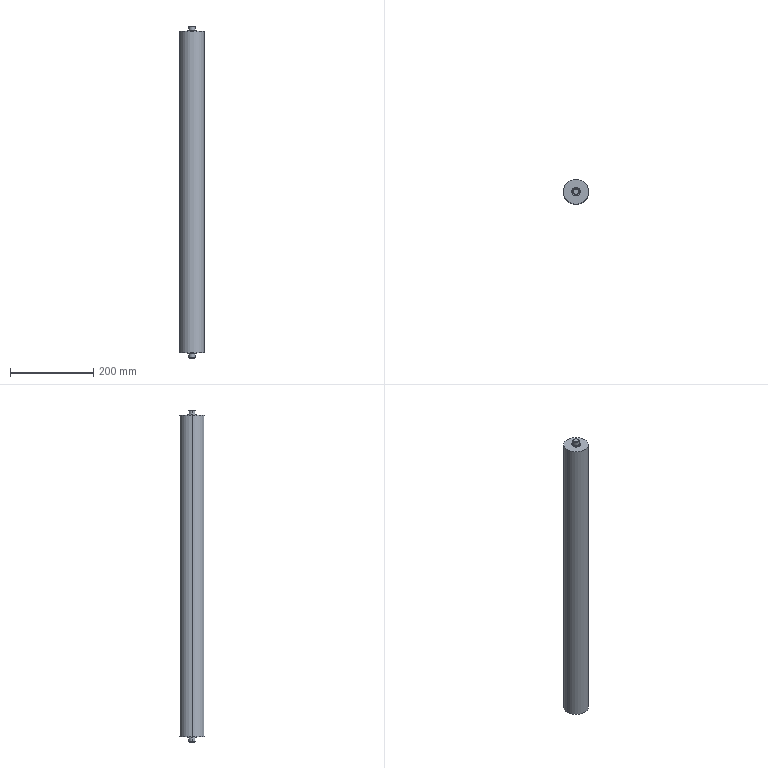Part | STEP file | Auxiliary roller 3 | 1 solid | 20 faces | box 60 x 60 x 799 mm | volume 2193510 mm3 | cylinder 10 | plane 6 | cone 4 | commonest cylinder face diameters 15 x4 20 x4 60 x2
STEP:
#1=CARTESIAN_POINT('',(0.,0.,0.));
#2=DIRECTION('',(0.,0.,1.));
#3=DIRECTION('',(1.,0.,0.));
#4=AXIS2_PLACEMENT_3D('',#1,#2,#3);
#5=CARTESIAN_POINT('',(30.,0.,0.));
#6=VERTEX_POINT('',#5);
#7=CARTESIAN_POINT('',(-30.,0.,0.));
#8=VERTEX_POINT('',#7);
#9=CARTESIAN_POINT('',(0.,0.,0.));
#10=DIRECTION('',(0.,0.,1.));
#11=DIRECTION('',(1.,0.,0.));
#12=AXIS2_PLACEMENT_3D('',#9,#10,#11);
#13=CIRCLE('',#12,30.);
#14=CARTESIAN_POINT('',(0.,0.,0.));
#15=DIRECTION('',(0.,0.,1.));
#16=DIRECTION('',(1.,0.,0.));
#17=AXIS2_PLACEMENT_3D('',#14,#15,#16);
#18=CYLINDRICAL_SURFACE('',#17,30.);
#19=CARTESIAN_POINT('',(0.,0.));
#20=DIRECTION('',(1.,0.));
#21=VECTOR('',#20,1.);
#22=LINE('',#19,#21);
#23=(GEOMETRIC_REPRESENTATION_CONTEXT(2)PARAMETRIC_REPRESENTATION_CONTEXT()REPRESENTATION_CONTEXT('',''));
#24=DEFINITIONAL_REPRESENTATION('',(#22),#23);
#25=PCURVE('',#18,#24);
#26=CARTESIAN_POINT('',(0.,0.,0.));
#27=DIRECTION('',(0.,0.,-1.));
#28=DIRECTION('',(-1.,0.,0.));
#29=AXIS2_PLACEMENT_3D('',#26,#27,#28);
#30=PLANE('',#29);
#31=CARTESIAN_POINT('',(-30.,0.));
#32=CARTESIAN_POINT('',(-30.,51.962));
#33=CARTESIAN_POINT('',(15.,25.981));
#34=CARTESIAN_POINT('',(60.,0.));
#35=CARTESIAN_POINT('',(15.,-25.981));
#36=CARTESIAN_POINT('',(-30.,-51.962));
#37=CARTESIAN_POINT('',(-30.,0.));
#38=(BOUNDED_CURVE()B_SPLINE_CURVE(2,(#31,#32,#33,#34,#35,#36,#37),.UNSPECIFIED.,.T.,.F.)B_SPLINE_CURVE_WITH_KNOTS((1,2,2,2,2,1),(-2.094,0.,2.094,4.189,6.283,8.378),.UNSPECIFIED.)CURVE()GEOMETRIC_REPRESENTATION_ITEM()RATIONAL_B_SPLINE_CURVE((1.,0.5,1.,0.5,1.,0.5,1.))REPRESENTATION_ITEM(''));
#39=(GEOMETRIC_REPRESENTATION_CONTEXT(2)PARAMETRIC_REPRESENTATION_CONTEXT()REPRESENTATION_CONTEXT('',''));
#40=DEFINITIONAL_REPRESENTATION('',(#38),#39);
#41=PCURVE('',#30,#40);
#42=SURFACE_CURVE('',#13,(#25,#41),.PCURVE_S1.);
#43=EDGE_CURVE('',#6,#8,#42,.T.);
#44=ORIENTED_EDGE('',*,*,#43,.T.);
#45=CARTESIAN_POINT('',(-30.,0.,774.));
#46=VERTEX_POINT('',#45);
#47=CARTESIAN_POINT('',(-30.,0.,0.));
#48=DIRECTION('',(0.,0.,1.));
#49=VECTOR('',#48,1.);
#50=LINE('',#47,#49);
#51=CARTESIAN_POINT('',(3.142,0.));
#52=DIRECTION('',(0.,1.));
#53=VECTOR('',#52,1.);
#54=LINE('',#51,#53);
#55=(GEOMETRIC_REPRESENTATION_CONTEXT(2)PARAMETRIC_REPRESENTATION_CONTEXT()REPRESENTATION_CONTEXT('',''));
#56=DEFINITIONAL_REPRESENTATION('',(#54),#55);
#57=PCURVE('',#18,#56);
#58=CARTESIAN_POINT('',(0.,0.,0.));
#59=DIRECTION('',(0.,0.,1.));
#60=DIRECTION('',(1.,0.,0.));
#61=AXIS2_PLACEMENT_3D('',#58,#59,#60);
#62=CYLINDRICAL_SURFACE('',#61,30.);
#63=CARTESIAN_POINT('',(3.142,0.));
#64=DIRECTION('',(0.,1.));
#65=VECTOR('',#64,1.);
#66=LINE('',#63,#65);
#67=(GEOMETRIC_REPRESENTATION_CONTEXT(2)PARAMETRIC_REPRESENTATION_CONTEXT()REPRESENTATION_CONTEXT('',''));
#68=DEFINITIONAL_REPRESENTATION('',(#66),#67);
#69=PCURVE('',#62,#68);
#70=SURFACE_CURVE('',#50,(#57,#69),.PCURVE_S1.);
#71=EDGE_CURVE('',#8,#46,#70,.T.);
#72=ORIENTED_EDGE('',*,*,#71,.T.);
#73=CARTESIAN_POINT('',(30.,0.,774.));
#74=VERTEX_POINT('',#73);
#75=CARTESIAN_POINT('',(0.,0.,774.));
#76=DIRECTION('',(0.,0.,-1.));
#77=DIRECTION('',(1.,0.,0.));
#78=AXIS2_PLACEMENT_3D('',#75,#76,#77);
#79=CIRCLE('',#78,30.);
#80=CARTESIAN_POINT('',(6.283,774.));
#81=DIRECTION('',(-1.,0.));
#82=VECTOR('',#81,1.);
#83=LINE('',#80,#82);
#84=(GEOMETRIC_REPRESENTATION_CONTEXT(2)PARAMETRIC_REPRESENTATION_CONTEXT()REPRESENTATION_CONTEXT('',''));
#85=DEFINITIONAL_REPRESENTATION('',(#83),#84);
#86=PCURVE('',#18,#85);
#87=CARTESIAN_POINT('',(0.,0.,774.));
#88=DIRECTION('',(0.,0.,-1.));
#89=DIRECTION('',(-1.,0.,0.));
#90=AXIS2_PLACEMENT_3D('',#87,#88,#89);
#91=PLANE('',#90);
#92=CARTESIAN_POINT('',(0.,0.));
#93=DIRECTION('',(-1.,0.));
#94=AXIS2_PLACEMENT_2D('',#92,#93);
#95=CIRCLE('',#94,30.);
#96=(GEOMETRIC_REPRESENTATION_CONTEXT(2)PARAMETRIC_REPRESENTATION_CONTEXT()REPRESENTATION_CONTEXT('',''));
#97=DEFINITIONAL_REPRESENTATION('',(#95),#96);
#98=PCURVE('',#91,#97);
#99=SURFACE_CURVE('',#79,(#86,#98),.PCURVE_S1.);
#100=EDGE_CURVE('',#46,#74,#99,.T.);
#101=ORIENTED_EDGE('',*,*,#100,.T.);
#102=CARTESIAN_POINT('',(30.,0.,0.));
#103=DIRECTION('',(0.,0.,1.));
#104=VECTOR('',#103,1.);
#105=LINE('',#102,#104);
#106=CARTESIAN_POINT('',(0.,0.));
#107=DIRECTION('',(0.,1.));
#108=VECTOR('',#107,1.);
#109=LINE('',#106,#108);
#110=(GEOMETRIC_REPRESENTATION_CONTEXT(2)PARAMETRIC_REPRESENTATION_CONTEXT()REPRESENTATION_CONTEXT('',''));
#111=DEFINITIONAL_REPRESENTATION('',(#109),#110);
#112=PCURVE('',#18,#111);
#113=CARTESIAN_POINT('',(6.283,0.));
#114=DIRECTION('',(0.,1.));
#115=VECTOR('',#114,1.);
#116=LINE('',#113,#115);
#117=(GEOMETRIC_REPRESENTATION_CONTEXT(2)PARAMETRIC_REPRESENTATION_CONTEXT()REPRESENTATION_CONTEXT('',''));
#118=DEFINITIONAL_REPRESENTATION('',(#116),#117);
#119=PCURVE('',#62,#118);
#120=SURFACE_CURVE('',#105,(#112,#119),.PCURVE_S1.);
#121=EDGE_CURVE('',#6,#74,#120,.T.);
#122=ORIENTED_EDGE('',*,*,#121,.F.);
#123=EDGE_LOOP('',(#44,#72,#101,#122));
#124=FACE_BOUND('',#123,.T.);
#125=ADVANCED_FACE('',(#124),#18,.T.);
#126=CARTESIAN_POINT('',(10.,0.,-2.5));
#127=VERTEX_POINT('',#126);
#128=CARTESIAN_POINT('',(-10.,0.,-2.5));
#129=VERTEX_POINT('',#128);
#130=CARTESIAN_POINT('',(0.,0.,-2.5));
#131=DIRECTION('',(0.,0.,1.));
#132=DIRECTION('',(1.,0.,0.));
#133=AXIS2_PLACEMENT_3D('',#130,#131,#132);
#134=CIRCLE('',#133,10.);
#135=CARTESIAN_POINT('',(0.,0.,0.));
#136=DIRECTION('',(0.,0.,1.));
#137=DIRECTION('',(1.,0.,0.));
#138=AXIS2_PLACEMENT_3D('',#135,#136,#137);
#139=CYLINDRICAL_SURFACE('',#138,10.);
#140=CARTESIAN_POINT('',(0.,-2.5));
#141=DIRECTION('',(1.,0.));
#142=VECTOR('',#141,1.);
#143=LINE('',#140,#142);
#144=(GEOMETRIC_REPRESENTATION_CONTEXT(2)PARAMETRIC_REPRESENTATION_CONTEXT()REPRESENTATION_CONTEXT('',''));
#145=DEFINITIONAL_REPRESENTATION('',(#143),#144);
#146=PCURVE('',#139,#145);
#147=CARTESIAN_POINT('',(0.,0.,-2.5));
#148=DIRECTION('',(0.,0.,-1.));
#149=DIRECTION('',(-1.,0.,0.));
#150=AXIS2_PLACEMENT_3D('',#147,#148,#149);
#151=PLANE('',#150);
#152=CARTESIAN_POINT('',(-10.,0.));
#153=CARTESIAN_POINT('',(-10.,17.321));
#154=CARTESIAN_POINT('',(5.,8.66));
#155=CARTESIAN_POINT('',(20.,0.));
#156=CARTESIAN_POINT('',(5.,-8.66));
#157=CARTESIAN_POINT('',(-10.,-17.321));
#158=CARTESIAN_POINT('',(-10.,0.));
#159=(BOUNDED_CURVE()B_SPLINE_CURVE(2,(#152,#153,#154,#155,#156,#157,#158),.UNSPECIFIED.,.T.,.F.)B_SPLINE_CURVE_WITH_KNOTS((1,2,2,2,2,1),(-2.094,0.,2.094,4.189,6.283,8.378),.UNSPECIFIED.)CURVE()GEOMETRIC_REPRESENTATION_ITEM()RATIONAL_B_SPLINE_CURVE((1.,0.5,1.,0.5,1.,0.5,1.))REPRESENTATION_ITEM(''));
#160=(GEOMETRIC_REPRESENTATION_CONTEXT(2)PARAMETRIC_REPRESENTATION_CONTEXT()REPRESENTATION_CONTEXT('',''));
#161=DEFINITIONAL_REPRESENTATION('',(#159),#160);
#162=PCURVE('',#151,#161);
#163=SURFACE_CURVE('',#134,(#146,#162),.PCURVE_S1.);
#164=EDGE_CURVE('',#127,#129,#163,.T.);
#165=ORIENTED_EDGE('',*,*,#164,.T.);
#166=CARTESIAN_POINT('',(-10.,0.,0.));
#167=VERTEX_POINT('',#166);
#168=CARTESIAN_POINT('',(-10.,0.,0.));
#169=DIRECTION('',(0.,0.,1.));
#170=VECTOR('',#169,1.);
#171=LINE('',#168,#170);
#172=CARTESIAN_POINT('',(3.142,0.));
#173=DIRECTION('',(0.,1.));
#174=VECTOR('',#173,1.);
#175=LINE('',#172,#174);
#176=(GEOMETRIC_REPRESENTATION_CONTEXT(2)PARAMETRIC_REPRESENTATION_CONTEXT()REPRESENTATION_CONTEXT('',''));
#177=DEFINITIONAL_REPRESENTATION('',(#175),#176);
#178=PCURVE('',#139,#177);
#179=CARTESIAN_POINT('',(0.,0.,0.));
#180=DIRECTION('',(0.,0.,1.));
#181=DIRECTION('',(1.,0.,0.));
#182=AXIS2_PLACEMENT_3D('',#179,#180,#181);
#183=CYLINDRICAL_SURFACE('',#182,10.);
#184=CARTESIAN_POINT('',(3.142,0.));
#185=DIRECTION('',(0.,1.));
#186=VECTOR('',#185,1.);
#187=LINE('',#184,#186);
#188=(GEOMETRIC_REPRESENTATION_CONTEXT(2)PARAMETRIC_REPRESENTATION_CONTEXT()REPRESENTATION_CONTEXT('',''));
#189=DEFINITIONAL_REPRESENTATION('',(#187),#188);
#190=PCURVE('',#183,#189);
#191=SURFACE_CURVE('',#171,(#178,#190),.PCURVE_S1.);
#192=EDGE_CURVE('',#129,#167,#191,.T.);
#193=ORIENTED_EDGE('',*,*,#192,.T.);
#194=CARTESIAN_POINT('',(10.,0.,0.));
#195=VERTEX_POINT('',#194);
#196=CARTESIAN_POINT('',(0.,0.,0.));
#197=DIRECTION('',(0.,0.,1.));
#198=DIRECTION('',(1.,0.,0.));
#199=AXIS2_PLACEMENT_3D('',#196,#197,#198);
#200=CIRCLE('',#199,10.);
#201=CARTESIAN_POINT('',(0.,0.));
#202=DIRECTION('',(1.,0.));
#203=VECTOR('',#202,1.);
#204=LINE('',#201,#203);
#205=(GEOMETRIC_REPRESENTATION_CONTEXT(2)PARAMETRIC_REPRESENTATION_CONTEXT()REPRESENTATION_CONTEXT('',''));
#206=DEFINITIONAL_REPRESENTATION('',(#204),#205);
#207=PCURVE('',#139,#206);
#208=CARTESIAN_POINT('',(-10.,0.));
#209=CARTESIAN_POINT('',(-10.,17.321));
#210=CARTESIAN_POINT('',(5.,8.66));
#211=CARTESIAN_POINT('',(20.,0.));
#212=CARTESIAN_POINT('',(5.,-8.66));
#213=CARTESIAN_POINT('',(-10.,-17.321));
#214=CARTESIAN_POINT('',(-10.,0.));
#215=(BOUNDED_CURVE()B_SPLINE_CURVE(2,(#208,#209,#210,#211,#212,#213,#214),.UNSPECIFIED.,.T.,.F.)B_SPLINE_CURVE_WITH_KNOTS((1,2,2,2,2,1),(-2.094,0.,2.094,4.189,6.283,8.378),.UNSPECIFIED.)CURVE()GEOMETRIC_REPRESENTATION_ITEM()RATIONAL_B_SPLINE_CURVE((1.,0.5,1.,0.5,1.,0.5,1.))REPRESENTATION_ITEM(''));
#216=(GEOMETRIC_REPRESENTATION_CONTEXT(2)PARAMETRIC_REPRESENTATION_CONTEXT()REPRESENTATION_CONTEXT('',''));
#217=DEFINITIONAL_REPRESENTATION('',(#215),#216);
#218=PCURVE('',#30,#217);
#219=SURFACE_CURVE('',#200,(#207,#218),.PCURVE_S1.);
#220=EDGE_CURVE('',#195,#167,#219,.T.);
#221=ORIENTED_EDGE('',*,*,#220,.F.);
#222=CARTESIAN_POINT('',(10.,0.,0.));
#223=DIRECTION('',(0.,0.,1.));
#224=VECTOR('',#223,1.);
#225=LINE('',#222,#224);
#226=CARTESIAN_POINT('',(0.,0.));
#227=DIRECTION('',(0.,1.));
#228=VECTOR('',#227,1.);
#229=LINE('',#226,#228);
#230=(GEOMETRIC_REPRESENTATION_CONTEXT(2)PARAMETRIC_REPRESENTATION_CONTEXT()REPRESENTATION_CONTEXT('',''));
#231=DEFINITIONAL_REPRESENTATION('',(#229),#230);
#232=PCURVE('',#139,#231);
#233=CARTESIAN_POINT('',(6.283,0.));
#234=DIRECTION('',(0.,1.));
#235=VECTOR('',#234,1.);
#236=LINE('',#233,#235);
#237=(GEOMETRIC_REPRESENTATION_CONTEXT(2)PARAMETRIC_REPRESENTATION_CONTEXT()REPRESENTATION_CONTEXT('',''));
#238=DEFINITIONAL_REPRESENTATION('',(#236),#237);
#239=PCURVE('',#183,#238);
#240=SURFACE_CURVE('',#225,(#232,#239),.PCURVE_S1.);
#241=EDGE_CURVE('',#127,#195,#240,.T.);
#242=ORIENTED_EDGE('',*,*,#241,.F.);
#243=EDGE_LOOP('',(#165,#193,#221,#242));
#244=FACE_BOUND('',#243,.T.);
#245=ADVANCED_FACE('',(#244),#139,.T.);
#246=CARTESIAN_POINT('',(10.,0.,774.));
#247=VERTEX_POINT('',#246);
#248=CARTESIAN_POINT('',(-10.,0.,774.));
#249=VERTEX_POINT('',#248);
#250=CARTESIAN_POINT('',(0.,0.,774.));
#251=DIRECTION('',(0.,0.,1.));
#252=DIRECTION('',(1.,0.,0.));
#253=AXIS2_PLACEMENT_3D('',#250,#251,#252);
#254=CIRCLE('',#253,10.);
#255=CARTESIAN_POINT('',(0.,0.,774.));
#256=DIRECTION('',(0.,0.,1.));
#257=DIRECTION('',(1.,0.,0.));
#258=AXIS2_PLACEMENT_3D('',#255,#256,#257);
#259=CYLINDRICAL_SURFACE('',#258,10.);
#260=CARTESIAN_POINT('',(0.,0.));
#261=DIRECTION('',(1.,0.));
#262=VECTOR('',#261,1.);
#263=LINE('',#260,#262);
#264=(GEOMETRIC_REPRESENTATION_CONTEXT(2)PARAMETRIC_REPRESENTATION_CONTEXT()REPRESENTATION_CONTEXT('',''));
#265=DEFINITIONAL_REPRESENTATION('',(#263),#264);
#266=PCURVE('',#259,#265);
#267=CARTESIAN_POINT('',(-10.,0.));
#268=CARTESIAN_POINT('',(-10.,17.321));
#269=CARTESIAN_POINT('',(5.,8.66));
#270=CARTESIAN_POINT('',(20.,0.));
#271=CARTESIAN_POINT('',(5.,-8.66));
#272=CARTESIAN_POINT('',(-10.,-17.321));
#273=CARTESIAN_POINT('',(-10.,0.));
#274=(BOUNDED_CURVE()B_SPLINE_CURVE(2,(#267,#268,#269,#270,#271,#272,#273),.UNSPECIFIED.,.T.,.F.)B_SPLINE_CURVE_WITH_KNOTS((1,2,2,2,2,1),(-2.094,0.,2.094,4.189,6.283,8.378),.UNSPECIFIED.)CURVE()GEOMETRIC_REPRESENTATION_ITEM()RATIONAL_B_SPLINE_CURVE((1.,0.5,1.,0.5,1.,0.5,1.))REPRESENTATION_ITEM(''));
#275=(GEOMETRIC_REPRESENTATION_CONTEXT(2)PARAMETRIC_REPRESENTATION_CONTEXT()REPRESENTATION_CONTEXT('',''));
#276=DEFINITIONAL_REPRESENTATION('',(#274),#275);
#277=PCURVE('',#91,#276);
#278=SURFACE_CURVE('',#254,(#266,#277),.PCURVE_S1.);
#279=EDGE_CURVE('',#247,#249,#278,.T.);
#280=ORIENTED_EDGE('',*,*,#279,.T.);
#281=CARTESIAN_POINT('',(-10.,0.,776.5));
#282=VERTEX_POINT('',#281);
#283=CARTESIAN_POINT('',(-10.,0.,774.));
#284=DIRECTION('',(0.,0.,1.));
#285=VECTOR('',#284,1.);
#286=LINE('',#283,#285);
#287=CARTESIAN_POINT('',(3.142,0.));
#288=DIRECTION('',(0.,1.));
#289=VECTOR('',#288,1.);
#290=LINE('',#287,#289);
#291=(GEOMETRIC_REPRESENTATION_CONTEXT(2)PARAMETRIC_REPRESENTATION_CONTEXT()REPRESENTATION_CONTEXT('',''));
#292=DEFINITIONAL_REPRESENTATION('',(#290),#291);
#293=PCURVE('',#259,#292);
#294=CARTESIAN_POINT('',(0.,0.,774.));
#295=DIRECTION('',(0.,0.,1.));
#296=DIRECTION('',(1.,0.,0.));
#297=AXIS2_PLACEMENT_3D('',#294,#295,#296);
#298=CYLINDRICAL_SURFACE('',#297,10.);
#299=CARTESIAN_POINT('',(3.142,0.));
#300=DIRECTION('',(0.,1.));
#301=VECTOR('',#300,1.);
#302=LINE('',#299,#301);
#303=(GEOMETRIC_REPRESENTATION_CONTEXT(2)PARAMETRIC_REPRESENTATION_CONTEXT()REPRESENTATION_CONTEXT('',''));
#304=DEFINITIONAL_REPRESENTATION('',(#302),#303);
#305=PCURVE('',#298,#304);
#306=SURFACE_CURVE('',#286,(#293,#305),.PCURVE_S1.);
#307=EDGE_CURVE('',#249,#282,#306,.T.);
#308=ORIENTED_EDGE('',*,*,#307,.T.);
#309=CARTESIAN_POINT('',(10.,0.,776.5));
#310=VERTEX_POINT('',#309);
#311=CARTESIAN_POINT('',(0.,0.,776.5));
#312=DIRECTION('',(0.,0.,-1.));
#313=DIRECTION('',(1.,0.,0.));
#314=AXIS2_PLACEMENT_3D('',#311,#312,#313);
#315=CIRCLE('',#314,10.);
#316=CARTESIAN_POINT('',(6.283,2.5));
#317=DIRECTION('',(-1.,0.));
#318=VECTOR('',#317,1.);
#319=LINE('',#316,#318);
#320=(GEOMETRIC_REPRESENTATION_CONTEXT(2)PARAMETRIC_REPRESENTATION_CONTEXT()REPRESENTATION_CONTEXT('',''));
#321=DEFINITIONAL_REPRESENTATION('',(#319),#320);
#322=PCURVE('',#259,#321);
#323=CARTESIAN_POINT('',(0.,0.,776.5));
#324=DIRECTION('',(0.,0.,-1.));
#325=DIRECTION('',(-1.,0.,0.));
#326=AXIS2_PLACEMENT_3D('',#323,#324,#325);
#327=PLANE('',#326);
#328=CARTESIAN_POINT('',(0.,0.));
#329=DIRECTION('',(-1.,0.));
#330=AXIS2_PLACEMENT_2D('',#328,#329);
#331=CIRCLE('',#330,10.);
#332=(GEOMETRIC_REPRESENTATION_CONTEXT(2)PARAMETRIC_REPRESENTATION_CONTEXT()REPRESENTATION_CONTEXT('',''));
#333=DEFINITIONAL_REPRESENTATION('',(#331),#332);
#334=PCURVE('',#327,#333);
#335=SURFACE_CURVE('',#315,(#322,#334),.PCURVE_S1.);
#336=EDGE_CURVE('',#282,#310,#335,.T.);
#337=ORIENTED_EDGE('',*,*,#336,.T.);
#338=CARTESIAN_POINT('',(10.,0.,774.));
#339=DIRECTION('',(0.,0.,1.));
#340=VECTOR('',#339,1.);
#341=LINE('',#338,#340);
#342=CARTESIAN_POINT('',(0.,0.));
#343=DIRECTION('',(0.,1.));
#344=VECTOR('',#343,1.);
#345=LINE('',#342,#344);
#346=(GEOMETRIC_REPRESENTATION_CONTEXT(2)PARAMETRIC_REPRESENTATION_CONTEXT()REPRESENTATION_CONTEXT('',''));
#347=DEFINITIONAL_REPRESENTATION('',(#345),#346);
#348=PCURVE('',#259,#347);
#349=CARTESIAN_POINT('',(6.283,0.));
#350=DIRECTION('',(0.,1.));
#351=VECTOR('',#350,1.);
#352=LINE('',#349,#351);
#353=(GEOMETRIC_REPRESENTATION_CONTEXT(2)PARAMETRIC_REPRESENTATION_CONTEXT()REPRESENTATION_CONTEXT('',''));
#354=DEFINITIONAL_REPRESENTATION('',(#352),#353);
#355=PCURVE('',#298,#354);
#356=SURFACE_CURVE('',#341,(#348,#355),.PCURVE_S1.);
#357=EDGE_CURVE('',#247,#310,#356,.T.);
#358=ORIENTED_EDGE('',*,*,#357,.F.);
#359=EDGE_LOOP('',(#280,#308,#337,#358));
#360=FACE_BOUND('',#359,.T.);
#361=ADVANCED_FACE('',(#360),#259,.T.);
#362=CARTESIAN_POINT('',(7.5,0.,-2.5));
#363=VERTEX_POINT('',#362);
#364=CARTESIAN_POINT('',(-7.5,0.,-2.5));
#365=VERTEX_POINT('',#364);
#366=CARTESIAN_POINT('',(0.,0.,-2.5));
#367=DIRECTION('',(0.,0.,1.));
#368=DIRECTION('',(-1.,0.,0.));
#369=AXIS2_PLACEMENT_3D('',#366,#367,#368);
#370=CIRCLE('',#369,7.5);
#371=CARTESIAN_POINT('',(0.,0.,-2.5));
#372=DIRECTION('',(0.,0.,-1.));
#373=DIRECTION('',(-1.,0.,0.));
#374=AXIS2_PLACEMENT_3D('',#371,#372,#373);
#375=CYLINDRICAL_SURFACE('',#374,7.5);
#376=CARTESIAN_POINT('',(6.283,0.));
#377=DIRECTION('',(-1.,0.));
#378=VECTOR('',#377,1.);
#379=LINE('',#376,#378);
#380=(GEOMETRIC_REPRESENTATION_CONTEXT(2)PARAMETRIC_REPRESENTATION_CONTEXT()REPRESENTATION_CONTEXT('',''));
#381=DEFINITIONAL_REPRESENTATION('',(#379),#380);
#382=PCURVE('',#375,#381);
#383=CARTESIAN_POINT('',(7.5,0.));
#384=CARTESIAN_POINT('',(7.5,-12.99));
#385=CARTESIAN_POINT('',(-3.75,-6.495));
#386=CARTESIAN_POINT('',(-15.,0.));
#387=CARTESIAN_POINT('',(-3.75,6.495));
#388=CARTESIAN_POINT('',(7.5,12.99));
#389=CARTESIAN_POINT('',(7.5,0.));
#390=(BOUNDED_CURVE()B_SPLINE_CURVE(2,(#383,#384,#385,#386,#387,#388,#389),.UNSPECIFIED.,.T.,.F.)B_SPLINE_CURVE_WITH_KNOTS((1,2,2,2,2,1),(-2.094,0.,2.094,4.189,6.283,8.378),.UNSPECIFIED.)CURVE()GEOMETRIC_REPRESENTATION_ITEM()RATIONAL_B_SPLINE_CURVE((1.,0.5,1.,0.5,1.,0.5,1.))REPRESENTATION_ITEM(''));
#391=(GEOMETRIC_REPRESENTATION_CONTEXT(2)PARAMETRIC_REPRESENTATION_CONTEXT()REPRESENTATION_CONTEXT('',''));
#392=DEFINITIONAL_REPRESENTATION('',(#390),#391);
#393=PCURVE('',#151,#392);
#394=SURFACE_CURVE('',#370,(#382,#393),.PCURVE_S1.);
#395=EDGE_CURVE('',#363,#365,#394,.T.);
#396=ORIENTED_EDGE('',*,*,#395,.F.);
#397=CARTESIAN_POINT('',(7.5,0.,-12.));
#398=VERTEX_POINT('',#397);
#399=CARTESIAN_POINT('',(7.5,0.,-2.5));
#400=DIRECTION('',(0.,0.,-1.));
#401=VECTOR('',#400,1.);
#402=LINE('',#399,#401);
#403=CARTESIAN_POINT('',(3.142,0.));
#404=DIRECTION('',(0.,1.));
#405=VECTOR('',#404,1.);
#406=LINE('',#403,#405);
#407=(GEOMETRIC_REPRESENTATION_CONTEXT(2)PARAMETRIC_REPRESENTATION_CONTEXT()REPRESENTATION_CONTEXT('',''));
#408=DEFINITIONAL_REPRESENTATION('',(#406),#407);
#409=PCURVE('',#375,#408);
#410=CARTESIAN_POINT('',(0.,0.,-2.5));
#411=DIRECTION('',(0.,0.,-1.));
#412=DIRECTION('',(-1.,0.,0.));
#413=AXIS2_PLACEMENT_3D('',#410,#411,#412);
#414=CYLINDRICAL_SURFACE('',#413,7.5);
#415=CARTESIAN_POINT('',(3.142,0.));
#416=DIRECTION('',(0.,1.));
#417=VECTOR('',#416,1.);
#418=LINE('',#415,#417);
#419=(GEOMETRIC_REPRESENTATION_CONTEXT(2)PARAMETRIC_REPRESENTATION_CONTEXT()REPRESENTATION_CONTEXT('',''));
#420=DEFINITIONAL_REPRESENTATION('',(#418),#419);
#421=PCURVE('',#414,#420);
#422=SURFACE_CURVE('',#402,(#409,#421),.PCURVE_S1.);
#423=EDGE_CURVE('',#363,#398,#422,.T.);
#424=ORIENTED_EDGE('',*,*,#423,.T.);
#425=CARTESIAN_POINT('',(-7.5,0.,-12.));
#426=VERTEX_POINT('',#425);
#427=CARTESIAN_POINT('',(0.,0.,-12.));
#428=DIRECTION('',(0.,0.,1.));
#429=DIRECTION('',(-1.,0.,0.));
#430=AXIS2_PLACEMENT_3D('',#427,#428,#429);
#431=CIRCLE('',#430,7.5);
#432=CARTESIAN_POINT('',(6.283,9.5));
#433=DIRECTION('',(-1.,0.));
#434=VECTOR('',#433,1.);
#435=LINE('',#432,#434);
#436=(GEOMETRIC_REPRESENTATION_CONTEXT(2)PARAMETRIC_REPRESENTATION_CONTEXT()REPRESENTATION_CONTEXT('',''));
#437=DEFINITIONAL_REPRESENTATION('',(#435),#436);
#438=PCURVE('',#375,#437);
#439=CARTESIAN_POINT('',(0.,0.,-12.));
#440=DIRECTION('',(0.,0.,1.));
#441=DIRECTION('',(1.,0.,0.));
#442=AXIS2_PLACEMENT_3D('',#439,#440,#441);
#443=CONICAL_SURFACE('',#442,7.5,0.7854);
#444=CARTESIAN_POINT('',(-3.142,0.));
#445=DIRECTION('',(1.,0.));
#446=VECTOR('',#445,1.);
#447=LINE('',#444,#446);
#448=(GEOMETRIC_REPRESENTATION_CONTEXT(2)PARAMETRIC_REPRESENTATION_CONTEXT()REPRESENTATION_CONTEXT('',''));
#449=DEFINITIONAL_REPRESENTATION('',(#447),#448);
#450=PCURVE('',#443,#449);
#451=SURFACE_CURVE('',#431,(#438,#450),.PCURVE_S1.);
#452=EDGE_CURVE('',#398,#426,#451,.T.);
#453=ORIENTED_EDGE('',*,*,#452,.T.);
#454=CARTESIAN_POINT('',(-7.5,0.,-2.5));
#455=DIRECTION('',(0.,0.,-1.));
#456=VECTOR('',#455,1.);
#457=LINE('',#454,#456);
#458=CARTESIAN_POINT('',(0.,0.));
#459=DIRECTION('',(0.,1.));
#460=VECTOR('',#459,1.);
#461=LINE('',#458,#460);
#462=(GEOMETRIC_REPRESENTATION_CONTEXT(2)PARAMETRIC_REPRESENTATION_CONTEXT()REPRESENTATION_CONTEXT('',''));
#463=DEFINITIONAL_REPRESENTATION('',(#461),#462);
#464=PCURVE('',#375,#463);
#465=CARTESIAN_POINT('',(6.283,0.));
#466=DIRECTION('',(0.,1.));
#467=VECTOR('',#466,1.);
#468=LINE('',#465,#467);
#469=(GEOMETRIC_REPRESENTATION_CONTEXT(2)PARAMETRIC_REPRESENTATION_CONTEXT()REPRESENTATION_CONTEXT('',''));
#470=DEFINITIONAL_REPRESENTATION('',(#468),#469);
#471=PCURVE('',#414,#470);
#472=SURFACE_CURVE('',#457,(#464,#471),.PCURVE_S1.);
#473=EDGE_CURVE('',#365,#426,#472,.T.);
#474=ORIENTED_EDGE('',*,*,#473,.F.);
#475=EDGE_LOOP('',(#396,#424,#453,#474));
#476=FACE_BOUND('',#475,.T.);
#477=ADVANCED_FACE('',(#476),#375,.T.);
#478=CARTESIAN_POINT('',(7.5,0.,776.5));
#479=VERTEX_POINT('',#478);
#480=CARTESIAN_POINT('',(-7.5,0.,776.5));
#481=VERTEX_POINT('',#480);
#482=CARTESIAN_POINT('',(0.,0.,776.5));
#483=DIRECTION('',(0.,0.,1.));
#484=DIRECTION('',(1.,0.,0.));
#485=AXIS2_PLACEMENT_3D('',#482,#483,#484);
#486=CIRCLE('',#485,7.5);
#487=CARTESIAN_POINT('',(0.,0.,776.5));
#488=DIRECTION('',(0.,0.,1.));
#489=DIRECTION('',(1.,0.,0.));
#490=AXIS2_PLACEMENT_3D('',#487,#488,#489);
#491=CYLINDRICAL_SURFACE('',#490,7.5);
#492=CARTESIAN_POINT('',(0.,0.));
#493=DIRECTION('',(1.,0.));
#494=VECTOR('',#493,1.);
#495=LINE('',#492,#494);
#496=(GEOMETRIC_REPRESENTATION_CONTEXT(2)PARAMETRIC_REPRESENTATION_CONTEXT()REPRESENTATION_CONTEXT('',''));
#497=DEFINITIONAL_REPRESENTATION('',(#495),#496);
#498=PCURVE('',#491,#497);
#499=CARTESIAN_POINT('',(-7.5,0.));
#500=CARTESIAN_POINT('',(-7.5,12.99));
#501=CARTESIAN_POINT('',(3.75,6.495));
#502=CARTESIAN_POINT('',(15.,0.));
#503=CARTESIAN_POINT('',(3.75,-6.495));
#504=CARTESIAN_POINT('',(-7.5,-12.99));
#505=CARTESIAN_POINT('',(-7.5,0.));
#506=(BOUNDED_CURVE()B_SPLINE_CURVE(2,(#499,#500,#501,#502,#503,#504,#505),.UNSPECIFIED.,.T.,.F.)B_SPLINE_CURVE_WITH_KNOTS((1,2,2,2,2,1),(-2.094,0.,2.094,4.189,6.283,8.378),.UNSPECIFIED.)CURVE()GEOMETRIC_REPRESENTATION_ITEM()RATIONAL_B_SPLINE_CURVE((1.,0.5,1.,0.5,1.,0.5,1.))REPRESENTATION_ITEM(''));
#507=(GEOMETRIC_REPRESENTATION_CONTEXT(2)PARAMETRIC_REPRESENTATION_CONTEXT()REPRESENTATION_CONTEXT('',''));
#508=DEFINITIONAL_REPRESENTATION('',(#506),#507);
#509=PCURVE('',#327,#508);
#510=SURFACE_CURVE('',#486,(#498,#509),.PCURVE_S1.);
#511=EDGE_CURVE('',#479,#481,#510,.T.);
#512=ORIENTED_EDGE('',*,*,#511,.T.);
#513=CARTESIAN_POINT('',(-7.5,0.,785.5));
#514=VERTEX_POINT('',#513);
#515=CARTESIAN_POINT('',(-7.5,0.,776.5));
#516=DIRECTION('',(0.,0.,1.));
#517=VECTOR('',#516,1.);
#518=LINE('',#515,#517);
#519=CARTESIAN_POINT('',(3.142,0.));
#520=DIRECTION('',(0.,1.));
#521=VECTOR('',#520,1.);
#522=LINE('',#519,#521);
#523=(GEOMETRIC_REPRESENTATION_CONTEXT(2)PARAMETRIC_REPRESENTATION_CONTEXT()REPRESENTATION_CONTEXT('',''));
#524=DEFINITIONAL_REPRESENTATION('',(#522),#523);
#525=PCURVE('',#491,#524);
#526=CARTESIAN_POINT('',(0.,0.,776.5));
#527=DIRECTION('',(0.,0.,1.));
#528=DIRECTION('',(1.,0.,0.));
#529=AXIS2_PLACEMENT_3D('',#526,#527,#528);
#530=CYLINDRICAL_SURFACE('',#529,7.5);
#531=CARTESIAN_POINT('',(3.142,0.));
#532=DIRECTION('',(0.,1.));
#533=VECTOR('',#532,1.);
#534=LINE('',#531,#533);
#535=(GEOMETRIC_REPRESENTATION_CONTEXT(2)PARAMETRIC_REPRESENTATION_CONTEXT()REPRESENTATION_CONTEXT('',''));
#536=DEFINITIONAL_REPRESENTATION('',(#534),#535);
#537=PCURVE('',#530,#536);
#538=SURFACE_CURVE('',#518,(#525,#537),.PCURVE_S1.);
#539=EDGE_CURVE('',#481,#514,#538,.T.);
#540=ORIENTED_EDGE('',*,*,#539,.T.);
#541=CARTESIAN_POINT('',(7.5,0.,785.5));
#542=VERTEX_POINT('',#541);
#543=CARTESIAN_POINT('',(0.,0.,785.5));
#544=DIRECTION('',(0.,0.,-1.));
#545=DIRECTION('',(1.,0.,0.));
#546=AXIS2_PLACEMENT_3D('',#543,#544,#545);
#547=CIRCLE('',#546,7.5);
#548=CARTESIAN_POINT('',(6.283,9.));
#549=DIRECTION('',(-1.,0.));
#550=VECTOR('',#549,1.);
#551=LINE('',#548,#550);
#552=(GEOMETRIC_REPRESENTATION_CONTEXT(2)PARAMETRIC_REPRESENTATION_CONTEXT()REPRESENTATION_CONTEXT('',''));
#553=DEFINITIONAL_REPRESENTATION('',(#551),#552);
#554=PCURVE('',#491,#553);
#555=CARTESIAN_POINT('',(0.,0.,785.5));
#556=DIRECTION('',(0.,0.,-1.));
#557=DIRECTION('',(-1.,0.,0.));
#558=AXIS2_PLACEMENT_3D('',#555,#556,#557);
#559=CONICAL_SURFACE('',#558,7.5,0.7854);
#560=CARTESIAN_POINT('',(-3.142,0.));
#561=DIRECTION('',(1.,0.));
#562=VECTOR('',#561,1.);
#563=LINE('',#560,#562);
#564=(GEOMETRIC_REPRESENTATION_CONTEXT(2)PARAMETRIC_REPRESENTATION_CONTEXT()REPRESENTATION_CONTEXT('',''));
#565=DEFINITIONAL_REPRESENTATION('',(#563),#564);
#566=PCURVE('',#559,#565);
#567=SURFACE_CURVE('',#547,(#554,#566),.PCURVE_S1.);
#568=EDGE_CURVE('',#514,#542,#567,.T.);
#569=ORIENTED_EDGE('',*,*,#568,.T.);
#570=CARTESIAN_POINT('',(7.5,0.,776.5));
#571=DIRECTION('',(0.,0.,1.));
#572=VECTOR('',#571,1.);
#573=LINE('',#570,#572);
#574=CARTESIAN_POINT('',(0.,0.));
#575=DIRECTION('',(0.,1.));
#576=VECTOR('',#575,1.);
#577=LINE('',#574,#576);
#578=(GEOMETRIC_REPRESENTATION_CONTEXT(2)PARAMETRIC_REPRESENTATION_CONTEXT()REPRESENTATION_CONTEXT('',''));
#579=DEFINITIONAL_REPRESENTATION('',(#577),#578);
#580=PCURVE('',#491,#579);
#581=CARTESIAN_POINT('',(6.283,0.));
#582=DIRECTION('',(0.,1.));
#583=VECTOR('',#582,1.);
#584=LINE('',#581,#583);
#585=(GEOMETRIC_REPRESENTATION_CONTEXT(2)PARAMETRIC_REPRESENTATION_CONTEXT()REPRESENTATION_CONTEXT('',''));
#586=DEFINITIONAL_REPRESENTATION('',(#584),#585);
#587=PCURVE('',#530,#586);
#588=SURFACE_CURVE('',#573,(#580,#587),.PCURVE_S1.);
#589=EDGE_CURVE('',#479,#542,#588,.T.);
#590=ORIENTED_EDGE('',*,*,#589,.F.);
#591=EDGE_LOOP('',(#512,#540,#569,#590));
#592=FACE_BOUND('',#591,.T.);
#593=ADVANCED_FACE('',(#592),#491,.T.);
#594=CARTESIAN_POINT('',(7.,0.,-12.5));
#595=VERTEX_POINT('',#594);
#596=CARTESIAN_POINT('',(-7.,0.,-12.5));
#597=VERTEX_POINT('',#596);
#598=CARTESIAN_POINT('',(0.,0.,-12.5));
#599=DIRECTION('',(0.,0.,1.));
#600=DIRECTION('',(1.,0.,0.));
#601=AXIS2_PLACEMENT_3D('',#598,#599,#600);
#602=CIRCLE('',#601,7.);
#603=CARTESIAN_POINT('',(0.,-0.5));
#604=DIRECTION('',(1.,0.));
#605=VECTOR('',#604,1.);
#606=LINE('',#603,#605);
#607=(GEOMETRIC_REPRESENTATION_CONTEXT(2)PARAMETRIC_REPRESENTATION_CONTEXT()REPRESENTATION_CONTEXT('',''));
#608=DEFINITIONAL_REPRESENTATION('',(#606),#607);
#609=PCURVE('',#443,#608);
#610=CARTESIAN_POINT('',(0.,0.,-12.5));
#611=DIRECTION('',(0.,0.,1.));
#612=DIRECTION('',(1.,0.,0.));
#613=AXIS2_PLACEMENT_3D('',#610,#611,#612);
#614=PLANE('',#613);
#615=CARTESIAN_POINT('',(0.,0.));
#616=DIRECTION('',(1.,0.));
#617=AXIS2_PLACEMENT_2D('',#615,#616);
#618=CIRCLE('',#617,7.);
#619=(GEOMETRIC_REPRESENTATION_CONTEXT(2)PARAMETRIC_REPRESENTATION_CONTEXT()REPRESENTATION_CONTEXT('',''));
#620=DEFINITIONAL_REPRESENTATION('',(#618),#619);
#621=PCURVE('',#614,#620);
#622=SURFACE_CURVE('',#602,(#609,#621),.PCURVE_S1.);
#623=EDGE_CURVE('',#595,#597,#622,.T.);
#624=ORIENTED_EDGE('',*,*,#623,.T.);
#625=CARTESIAN_POINT('',(-7.5,0.,-12.));
#626=DIRECTION('',(-0.7071,0.,0.7071));
#627=VECTOR('',#626,1.);
#628=LINE('',#625,#627);
#629=CARTESIAN_POINT('',(3.142,0.));
#630=DIRECTION('',(0.,1.));
#631=VECTOR('',#630,1.);
#632=LINE('',#629,#631);
#633=(GEOMETRIC_REPRESENTATION_CONTEXT(2)PARAMETRIC_REPRESENTATION_CONTEXT()REPRESENTATION_CONTEXT('',''));
#634=DEFINITIONAL_REPRESENTATION('',(#632),#633);
#635=PCURVE('',#443,#634);
#636=CARTESIAN_POINT('',(0.,0.,-12.));
#637=DIRECTION('',(0.,0.,1.));
#638=DIRECTION('',(1.,0.,0.));
#639=AXIS2_PLACEMENT_3D('',#636,#637,#638);
#640=CONICAL_SURFACE('',#639,7.5,0.7854);
#641=CARTESIAN_POINT('',(3.142,0.));
#642=DIRECTION('',(0.,1.));
#643=VECTOR('',#642,1.);
#644=LINE('',#641,#643);
#645=(GEOMETRIC_REPRESENTATION_CONTEXT(2)PARAMETRIC_REPRESENTATION_CONTEXT()REPRESENTATION_CONTEXT('',''));
#646=DEFINITIONAL_REPRESENTATION('',(#644),#645);
#647=PCURVE('',#640,#646);
#648=SURFACE_CURVE('',#628,(#635,#647),.PCURVE_S1.);
#649=EDGE_CURVE('',#597,#426,#648,.T.);
#650=ORIENTED_EDGE('',*,*,#649,.T.);
#651=ORIENTED_EDGE('',*,*,#452,.F.);
#652=CARTESIAN_POINT('',(7.5,0.,-12.));
#653=DIRECTION('',(0.7071,0.,0.7071));
#654=VECTOR('',#653,1.);
#655=LINE('',#652,#654);
#656=CARTESIAN_POINT('',(0.,0.));
#657=DIRECTION('',(0.,1.));
#658=VECTOR('',#657,1.);
#659=LINE('',#656,#658);
#660=(GEOMETRIC_REPRESENTATION_CONTEXT(2)PARAMETRIC_REPRESENTATION_CONTEXT()REPRESENTATION_CONTEXT('',''));
#661=DEFINITIONAL_REPRESENTATION('',(#659),#660);
#662=PCURVE('',#443,#661);
#663=CARTESIAN_POINT('',(6.283,0.));
#664=DIRECTION('',(0.,1.));
#665=VECTOR('',#664,1.);
#666=LINE('',#663,#665);
#667=(GEOMETRIC_REPRESENTATION_CONTEXT(2)PARAMETRIC_REPRESENTATION_CONTEXT()REPRESENTATION_CONTEXT('',''));
#668=DEFINITIONAL_REPRESENTATION('',(#666),#667);
#669=PCURVE('',#640,#668);
#670=SURFACE_CURVE('',#655,(#662,#669),.PCURVE_S1.);
#671=EDGE_CURVE('',#595,#398,#670,.T.);
#672=ORIENTED_EDGE('',*,*,#671,.F.);
#673=EDGE_LOOP('',(#624,#650,#651,#672));
#674=FACE_BOUND('',#673,.T.);
#675=ADVANCED_FACE('',(#674),#443,.T.);
#676=CARTESIAN_POINT('',(-6.5,0.,786.5));
#677=VERTEX_POINT('',#676);
#678=CARTESIAN_POINT('',(6.5,0.,786.5));
#679=VERTEX_POINT('',#678);
#680=CARTESIAN_POINT('',(0.,0.,786.5));
#681=DIRECTION('',(0.,0.,-1.));
#682=DIRECTION('',(-1.,0.,0.));
#683=AXIS2_PLACEMENT_3D('',#680,#681,#682);
#684=CIRCLE('',#683,6.5);
#685=CARTESIAN_POINT('',(0.,-1.));
#686=DIRECTION('',(1.,0.));
#687=VECTOR('',#686,1.);
#688=LINE('',#685,#687);
#689=(GEOMETRIC_REPRESENTATION_CONTEXT(2)PARAMETRIC_REPRESENTATION_CONTEXT()REPRESENTATION_CONTEXT('',''));
#690=DEFINITIONAL_REPRESENTATION('',(#688),#689);
#691=PCURVE('',#559,#690);
#692=CARTESIAN_POINT('',(0.,0.,786.5));
#693=DIRECTION('',(0.,0.,-1.));
#694=DIRECTION('',(-1.,0.,0.));
#695=AXIS2_PLACEMENT_3D('',#692,#693,#694);
#696=PLANE('',#695);
#697=CARTESIAN_POINT('',(0.,0.));
#698=DIRECTION('',(1.,0.));
#699=AXIS2_PLACEMENT_2D('',#697,#698);
#700=CIRCLE('',#699,6.5);
#701=(GEOMETRIC_REPRESENTATION_CONTEXT(2)PARAMETRIC_REPRESENTATION_CONTEXT()REPRESENTATION_CONTEXT('',''));
#702=DEFINITIONAL_REPRESENTATION('',(#700),#701);
#703=PCURVE('',#696,#702);
#704=SURFACE_CURVE('',#684,(#691,#703),.PCURVE_S1.);
#705=EDGE_CURVE('',#677,#679,#704,.T.);
#706=ORIENTED_EDGE('',*,*,#705,.T.);
#707=CARTESIAN_POINT('',(7.5,0.,785.5));
#708=DIRECTION('',(0.7071,0.,-0.7071));
#709=VECTOR('',#708,1.);
#710=LINE('',#707,#709);
#711=CARTESIAN_POINT('',(3.142,0.));
#712=DIRECTION('',(0.,1.));
#713=VECTOR('',#712,1.);
#714=LINE('',#711,#713);
#715=(GEOMETRIC_REPRESENTATION_CONTEXT(2)PARAMETRIC_REPRESENTATION_CONTEXT()REPRESENTATION_CONTEXT('',''));
#716=DEFINITIONAL_REPRESENTATION('',(#714),#715);
#717=PCURVE('',#559,#716);
#718=CARTESIAN_POINT('',(0.,0.,785.5));
#719=DIRECTION('',(0.,0.,-1.));
#720=DIRECTION('',(-1.,0.,0.));
#721=AXIS2_PLACEMENT_3D('',#718,#719,#720);
#722=CONICAL_SURFACE('',#721,7.5,0.7854);
#723=CARTESIAN_POINT('',(3.142,0.));
#724=DIRECTION('',(0.,1.));
#725=VECTOR('',#724,1.);
#726=LINE('',#723,#725);
#727=(GEOMETRIC_REPRESENTATION_CONTEXT(2)PARAMETRIC_REPRESENTATION_CONTEXT()REPRESENTATION_CONTEXT('',''));
#728=DEFINITIONAL_REPRESENTATION('',(#726),#727);
#729=PCURVE('',#722,#728);
#730=SURFACE_CURVE('',#710,(#717,#729),.PCURVE_S1.);
#731=EDGE_CURVE('',#679,#542,#730,.T.);
#732=ORIENTED_EDGE('',*,*,#731,.T.);
#733=ORIENTED_EDGE('',*,*,#568,.F.);
#734=CARTESIAN_POINT('',(-7.5,0.,785.5));
#735=DIRECTION('',(-0.7071,0.,-0.7071));
#736=VECTOR('',#735,1.);
#737=LINE('',#734,#736);
#738=CARTESIAN_POINT('',(0.,0.));
#739=DIRECTION('',(0.,1.));
#740=VECTOR('',#739,1.);
#741=LINE('',#738,#740);
#742=(GEOMETRIC_REPRESENTATION_CONTEXT(2)PARAMETRIC_REPRESENTATION_CONTEXT()REPRESENTATION_CONTEXT('',''));
#743=DEFINITIONAL_REPRESENTATION('',(#741),#742);
#744=PCURVE('',#559,#743);
#745=CARTESIAN_POINT('',(6.283,0.));
#746=DIRECTION('',(0.,1.));
#747=VECTOR('',#746,1.);
#748=LINE('',#745,#747);
#749=(GEOMETRIC_REPRESENTATION_CONTEXT(2)PARAMETRIC_REPRESENTATION_CONTEXT()REPRESENTATION_CONTEXT('',''));
#750=DEFINITIONAL_REPRESENTATION('',(#748),#749);
#751=PCURVE('',#722,#750);
#752=SURFACE_CURVE('',#737,(#744,#751),.PCURVE_S1.);
#753=EDGE_CURVE('',#677,#514,#752,.T.);
#754=ORIENTED_EDGE('',*,*,#753,.F.);
#755=EDGE_LOOP('',(#706,#732,#733,#754));
#756=FACE_BOUND('',#755,.T.);
#757=ADVANCED_FACE('',(#756),#559,.T.);
#758=ORIENTED_EDGE('',*,*,#71,.F.);
#759=CARTESIAN_POINT('',(0.,0.,0.));
#760=DIRECTION('',(0.,0.,1.));
#761=DIRECTION('',(1.,0.,0.));
#762=AXIS2_PLACEMENT_3D('',#759,#760,#761);
#763=CIRCLE('',#762,30.);
#764=CARTESIAN_POINT('',(0.,0.));
#765=DIRECTION('',(1.,0.));
#766=VECTOR('',#765,1.);
#767=LINE('',#764,#766);
#768=(GEOMETRIC_REPRESENTATION_CONTEXT(2)PARAMETRIC_REPRESENTATION_CONTEXT()REPRESENTATION_CONTEXT('',''));
#769=DEFINITIONAL_REPRESENTATION('',(#767),#768);
#770=PCURVE('',#62,#769);
#771=CARTESIAN_POINT('',(-30.,0.));
#772=CARTESIAN_POINT('',(-30.,51.962));
#773=CARTESIAN_POINT('',(15.,25.981));
#774=CARTESIAN_POINT('',(60.,0.));
#775=CARTESIAN_POINT('',(15.,-25.981));
#776=CARTESIAN_POINT('',(-30.,-51.962));
#777=CARTESIAN_POINT('',(-30.,0.));
#778=(BOUNDED_CURVE()B_SPLINE_CURVE(2,(#771,#772,#773,#774,#775,#776,#777),.UNSPECIFIED.,.T.,.F.)B_SPLINE_CURVE_WITH_KNOTS((1,2,2,2,2,1),(-2.094,0.,2.094,4.189,6.283,8.378),.UNSPECIFIED.)CURVE()GEOMETRIC_REPRESENTATION_ITEM()RATIONAL_B_SPLINE_CURVE((1.,0.5,1.,0.5,1.,0.5,1.))REPRESENTATION_ITEM(''));
#779=(GEOMETRIC_REPRESENTATION_CONTEXT(2)PARAMETRIC_REPRESENTATION_CONTEXT()REPRESENTATION_CONTEXT('',''));
#780=DEFINITIONAL_REPRESENTATION('',(#778),#779);
#781=PCURVE('',#30,#780);
#782=SURFACE_CURVE('',#763,(#770,#781),.PCURVE_S1.);
#783=EDGE_CURVE('',#8,#6,#782,.T.);
#784=ORIENTED_EDGE('',*,*,#783,.T.);
#785=ORIENTED_EDGE('',*,*,#121,.T.);
#786=CARTESIAN_POINT('',(0.,0.,774.));
#787=DIRECTION('',(0.,0.,-1.));
#788=DIRECTION('',(1.,0.,0.));
#789=AXIS2_PLACEMENT_3D('',#786,#787,#788);
#790=CIRCLE('',#789,30.);
#791=CARTESIAN_POINT('',(6.283,774.));
#792=DIRECTION('',(-1.,0.));
#793=VECTOR('',#792,1.);
#794=LINE('',#791,#793);
#795=(GEOMETRIC_REPRESENTATION_CONTEXT(2)PARAMETRIC_REPRESENTATION_CONTEXT()REPRESENTATION_CONTEXT('',''));
#796=DEFINITIONAL_REPRESENTATION('',(#794),#795);
#797=PCURVE('',#62,#796);
#798=CARTESIAN_POINT('',(0.,0.));
#799=DIRECTION('',(-1.,0.));
#800=AXIS2_PLACEMENT_2D('',#798,#799);
#801=CIRCLE('',#800,30.);
#802=(GEOMETRIC_REPRESENTATION_CONTEXT(2)PARAMETRIC_REPRESENTATION_CONTEXT()REPRESENTATION_CONTEXT('',''));
#803=DEFINITIONAL_REPRESENTATION('',(#801),#802);
#804=PCURVE('',#91,#803);
#805=SURFACE_CURVE('',#790,(#797,#804),.PCURVE_S1.);
#806=EDGE_CURVE('',#74,#46,#805,.T.);
#807=ORIENTED_EDGE('',*,*,#806,.T.);
#808=EDGE_LOOP('',(#758,#784,#785,#807));
#809=FACE_BOUND('',#808,.T.);
#810=ADVANCED_FACE('',(#809),#62,.T.);
#811=ORIENTED_EDGE('',*,*,#220,.T.);
#812=CARTESIAN_POINT('',(0.,0.,0.));
#813=DIRECTION('',(0.,0.,1.));
#814=DIRECTION('',(1.,0.,0.));
#815=AXIS2_PLACEMENT_3D('',#812,#813,#814);
#816=CIRCLE('',#815,10.);
#817=CARTESIAN_POINT('',(-10.,0.));
#818=CARTESIAN_POINT('',(-10.,17.321));
#819=CARTESIAN_POINT('',(5.,8.66));
#820=CARTESIAN_POINT('',(20.,0.));
#821=CARTESIAN_POINT('',(5.,-8.66));
#822=CARTESIAN_POINT('',(-10.,-17.321));
#823=CARTESIAN_POINT('',(-10.,0.));
#824=(BOUNDED_CURVE()B_SPLINE_CURVE(2,(#817,#818,#819,#820,#821,#822,#823),.UNSPECIFIED.,.T.,.F.)B_SPLINE_CURVE_WITH_KNOTS((1,2,2,2,2,1),(-2.094,0.,2.094,4.189,6.283,8.378),.UNSPECIFIED.)CURVE()GEOMETRIC_REPRESENTATION_ITEM()RATIONAL_B_SPLINE_CURVE((1.,0.5,1.,0.5,1.,0.5,1.))REPRESENTATION_ITEM(''));
#825=(GEOMETRIC_REPRESENTATION_CONTEXT(2)PARAMETRIC_REPRESENTATION_CONTEXT()REPRESENTATION_CONTEXT('',''));
#826=DEFINITIONAL_REPRESENTATION('',(#824),#825);
#827=PCURVE('',#30,#826);
#828=CARTESIAN_POINT('',(0.,0.));
#829=DIRECTION('',(1.,0.));
#830=VECTOR('',#829,1.);
#831=LINE('',#828,#830);
#832=(GEOMETRIC_REPRESENTATION_CONTEXT(2)PARAMETRIC_REPRESENTATION_CONTEXT()REPRESENTATION_CONTEXT('',''));
#833=DEFINITIONAL_REPRESENTATION('',(#831),#832);
#834=PCURVE('',#183,#833);
#835=SURFACE_CURVE('',#816,(#827,#834),.PCURVE_S1.);
#836=EDGE_CURVE('',#167,#195,#835,.T.);
#837=ORIENTED_EDGE('',*,*,#836,.T.);
#838=EDGE_LOOP('',(#811,#837));
#839=FACE_BOUND('',#838,.T.);
#840=ORIENTED_EDGE('',*,*,#43,.F.);
#841=ORIENTED_EDGE('',*,*,#783,.F.);
#842=EDGE_LOOP('',(#840,#841));
#843=FACE_BOUND('',#842,.T.);
#844=ADVANCED_FACE('',(#839,#843),#30,.T.);
#845=ORIENTED_EDGE('',*,*,#279,.F.);
#846=CARTESIAN_POINT('',(0.,0.,774.));
#847=DIRECTION('',(0.,0.,1.));
#848=DIRECTION('',(1.,0.,0.));
#849=AXIS2_PLACEMENT_3D('',#846,#847,#848);
#850=CIRCLE('',#849,10.);
#851=CARTESIAN_POINT('',(-10.,0.));
#852=CARTESIAN_POINT('',(-10.,17.321));
#853=CARTESIAN_POINT('',(5.,8.66));
#854=CARTESIAN_POINT('',(20.,0.));
#855=CARTESIAN_POINT('',(5.,-8.66));
#856=CARTESIAN_POINT('',(-10.,-17.321));
#857=CARTESIAN_POINT('',(-10.,0.));
#858=(BOUNDED_CURVE()B_SPLINE_CURVE(2,(#851,#852,#853,#854,#855,#856,#857),.UNSPECIFIED.,.T.,.F.)B_SPLINE_CURVE_WITH_KNOTS((1,2,2,2,2,1),(-2.094,0.,2.094,4.189,6.283,8.378),.UNSPECIFIED.)CURVE()GEOMETRIC_REPRESENTATION_ITEM()RATIONAL_B_SPLINE_CURVE((1.,0.5,1.,0.5,1.,0.5,1.))REPRESENTATION_ITEM(''));
#859=(GEOMETRIC_REPRESENTATION_CONTEXT(2)PARAMETRIC_REPRESENTATION_CONTEXT()REPRESENTATION_CONTEXT('',''));
#860=DEFINITIONAL_REPRESENTATION('',(#858),#859);
#861=PCURVE('',#91,#860);
#862=CARTESIAN_POINT('',(0.,0.));
#863=DIRECTION('',(1.,0.));
#864=VECTOR('',#863,1.);
#865=LINE('',#862,#864);
#866=(GEOMETRIC_REPRESENTATION_CONTEXT(2)PARAMETRIC_REPRESENTATION_CONTEXT()REPRESENTATION_CONTEXT('',''));
#867=DEFINITIONAL_REPRESENTATION('',(#865),#866);
#868=PCURVE('',#298,#867);
#869=SURFACE_CURVE('',#850,(#861,#868),.PCURVE_S1.);
#870=EDGE_CURVE('',#249,#247,#869,.T.);
#871=ORIENTED_EDGE('',*,*,#870,.F.);
#872=EDGE_LOOP('',(#845,#871));
#873=FACE_BOUND('',#872,.T.);
#874=ORIENTED_EDGE('',*,*,#806,.F.);
#875=ORIENTED_EDGE('',*,*,#100,.F.);
#876=EDGE_LOOP('',(#874,#875));
#877=FACE_BOUND('',#876,.T.);
#878=ADVANCED_FACE('',(#873,#877),#91,.F.);
#879=ORIENTED_EDGE('',*,*,#192,.F.);
#880=CARTESIAN_POINT('',(0.,0.,-2.5));
#881=DIRECTION('',(0.,0.,1.));
#882=DIRECTION('',(1.,0.,0.));
#883=AXIS2_PLACEMENT_3D('',#880,#881,#882);
#884=CIRCLE('',#883,10.);
#885=CARTESIAN_POINT('',(0.,-2.5));
#886=DIRECTION('',(1.,0.));
#887=VECTOR('',#886,1.);
#888=LINE('',#885,#887);
#889=(GEOMETRIC_REPRESENTATION_CONTEXT(2)PARAMETRIC_REPRESENTATION_CONTEXT()REPRESENTATION_CONTEXT('',''));
#890=DEFINITIONAL_REPRESENTATION('',(#888),#889);
#891=PCURVE('',#183,#890);
#892=CARTESIAN_POINT('',(-10.,0.));
#893=CARTESIAN_POINT('',(-10.,17.321));
#894=CARTESIAN_POINT('',(5.,8.66));
#895=CARTESIAN_POINT('',(20.,0.));
#896=CARTESIAN_POINT('',(5.,-8.66));
#897=CARTESIAN_POINT('',(-10.,-17.321));
#898=CARTESIAN_POINT('',(-10.,0.));
#899=(BOUNDED_CURVE()B_SPLINE_CURVE(2,(#892,#893,#894,#895,#896,#897,#898),.UNSPECIFIED.,.T.,.F.)B_SPLINE_CURVE_WITH_KNOTS((1,2,2,2,2,1),(-2.094,0.,2.094,4.189,6.283,8.378),.UNSPECIFIED.)CURVE()GEOMETRIC_REPRESENTATION_ITEM()RATIONAL_B_SPLINE_CURVE((1.,0.5,1.,0.5,1.,0.5,1.))REPRESENTATION_ITEM(''));
#900=(GEOMETRIC_REPRESENTATION_CONTEXT(2)PARAMETRIC_REPRESENTATION_CONTEXT()REPRESENTATION_CONTEXT('',''));
#901=DEFINITIONAL_REPRESENTATION('',(#899),#900);
#902=PCURVE('',#151,#901);
#903=SURFACE_CURVE('',#884,(#891,#902),.PCURVE_S1.);
#904=EDGE_CURVE('',#129,#127,#903,.T.);
#905=ORIENTED_EDGE('',*,*,#904,.T.);
#906=ORIENTED_EDGE('',*,*,#241,.T.);
#907=ORIENTED_EDGE('',*,*,#836,.F.);
#908=EDGE_LOOP('',(#879,#905,#906,#907));
#909=FACE_BOUND('',#908,.T.);
#910=ADVANCED_FACE('',(#909),#183,.T.);
#911=ORIENTED_EDGE('',*,*,#307,.F.);
#912=ORIENTED_EDGE('',*,*,#870,.T.);
#913=ORIENTED_EDGE('',*,*,#357,.T.);
#914=CARTESIAN_POINT('',(0.,0.,776.5));
#915=DIRECTION('',(0.,0.,-1.));
#916=DIRECTION('',(1.,0.,0.));
#917=AXIS2_PLACEMENT_3D('',#914,#915,#916);
#918=CIRCLE('',#917,10.);
#919=CARTESIAN_POINT('',(6.283,2.5));
#920=DIRECTION('',(-1.,0.));
#921=VECTOR('',#920,1.);
#922=LINE('',#919,#921);
#923=(GEOMETRIC_REPRESENTATION_CONTEXT(2)PARAMETRIC_REPRESENTATION_CONTEXT()REPRESENTATION_CONTEXT('',''));
#924=DEFINITIONAL_REPRESENTATION('',(#922),#923);
#925=PCURVE('',#298,#924);
#926=CARTESIAN_POINT('',(0.,0.));
#927=DIRECTION('',(-1.,0.));
#928=AXIS2_PLACEMENT_2D('',#926,#927);
#929=CIRCLE('',#928,10.);
#930=(GEOMETRIC_REPRESENTATION_CONTEXT(2)PARAMETRIC_REPRESENTATION_CONTEXT()REPRESENTATION_CONTEXT('',''));
#931=DEFINITIONAL_REPRESENTATION('',(#929),#930);
#932=PCURVE('',#327,#931);
#933=SURFACE_CURVE('',#918,(#925,#932),.PCURVE_S1.);
#934=EDGE_CURVE('',#310,#282,#933,.T.);
#935=ORIENTED_EDGE('',*,*,#934,.T.);
#936=EDGE_LOOP('',(#911,#912,#913,#935));
#937=FACE_BOUND('',#936,.T.);
#938=ADVANCED_FACE('',(#937),#298,.T.);
#939=CARTESIAN_POINT('',(0.,0.,-2.5));
#940=DIRECTION('',(0.,0.,1.));
#941=DIRECTION('',(-1.,0.,0.));
#942=AXIS2_PLACEMENT_3D('',#939,#940,#941);
#943=CIRCLE('',#942,7.5);
#944=CARTESIAN_POINT('',(7.5,0.));
#945=CARTESIAN_POINT('',(7.5,-12.99));
#946=CARTESIAN_POINT('',(-3.75,-6.495));
#947=CARTESIAN_POINT('',(-15.,0.));
#948=CARTESIAN_POINT('',(-3.75,6.495));
#949=CARTESIAN_POINT('',(7.5,12.99));
#950=CARTESIAN_POINT('',(7.5,0.));
#951=(BOUNDED_CURVE()B_SPLINE_CURVE(2,(#944,#945,#946,#947,#948,#949,#950),.UNSPECIFIED.,.T.,.F.)B_SPLINE_CURVE_WITH_KNOTS((1,2,2,2,2,1),(-2.094,0.,2.094,4.189,6.283,8.378),.UNSPECIFIED.)CURVE()GEOMETRIC_REPRESENTATION_ITEM()RATIONAL_B_SPLINE_CURVE((1.,0.5,1.,0.5,1.,0.5,1.))REPRESENTATION_ITEM(''));
#952=(GEOMETRIC_REPRESENTATION_CONTEXT(2)PARAMETRIC_REPRESENTATION_CONTEXT()REPRESENTATION_CONTEXT('',''));
#953=DEFINITIONAL_REPRESENTATION('',(#951),#952);
#954=PCURVE('',#151,#953);
#955=CARTESIAN_POINT('',(6.283,0.));
#956=DIRECTION('',(-1.,0.));
#957=VECTOR('',#956,1.);
#958=LINE('',#955,#957);
#959=(GEOMETRIC_REPRESENTATION_CONTEXT(2)PARAMETRIC_REPRESENTATION_CONTEXT()REPRESENTATION_CONTEXT('',''));
#960=DEFINITIONAL_REPRESENTATION('',(#958),#959);
#961=PCURVE('',#414,#960);
#962=SURFACE_CURVE('',#943,(#954,#961),.PCURVE_S1.);
#963=EDGE_CURVE('',#365,#363,#962,.T.);
#964=ORIENTED_EDGE('',*,*,#963,.T.);
#965=ORIENTED_EDGE('',*,*,#395,.T.);
#966=EDGE_LOOP('',(#964,#965));
#967=FACE_BOUND('',#966,.T.);
#968=ORIENTED_EDGE('',*,*,#164,.F.);
#969=ORIENTED_EDGE('',*,*,#904,.F.);
#970=EDGE_LOOP('',(#968,#969));
#971=FACE_BOUND('',#970,.T.);
#972=ADVANCED_FACE('',(#967,#971),#151,.T.);
#973=ORIENTED_EDGE('',*,*,#511,.F.);
#974=CARTESIAN_POINT('',(0.,0.,776.5));
#975=DIRECTION('',(0.,0.,1.));
#976=DIRECTION('',(1.,0.,0.));
#977=AXIS2_PLACEMENT_3D('',#974,#975,#976);
#978=CIRCLE('',#977,7.5);
#979=CARTESIAN_POINT('',(-7.5,0.));
#980=CARTESIAN_POINT('',(-7.5,12.99));
#981=CARTESIAN_POINT('',(3.75,6.495));
#982=CARTESIAN_POINT('',(15.,0.));
#983=CARTESIAN_POINT('',(3.75,-6.495));
#984=CARTESIAN_POINT('',(-7.5,-12.99));
#985=CARTESIAN_POINT('',(-7.5,0.));
#986=(BOUNDED_CURVE()B_SPLINE_CURVE(2,(#979,#980,#981,#982,#983,#984,#985),.UNSPECIFIED.,.T.,.F.)B_SPLINE_CURVE_WITH_KNOTS((1,2,2,2,2,1),(-2.094,0.,2.094,4.189,6.283,8.378),.UNSPECIFIED.)CURVE()GEOMETRIC_REPRESENTATION_ITEM()RATIONAL_B_SPLINE_CURVE((1.,0.5,1.,0.5,1.,0.5,1.))REPRESENTATION_ITEM(''));
#987=(GEOMETRIC_REPRESENTATION_CONTEXT(2)PARAMETRIC_REPRESENTATION_CONTEXT()REPRESENTATION_CONTEXT('',''));
#988=DEFINITIONAL_REPRESENTATION('',(#986),#987);
#989=PCURVE('',#327,#988);
#990=CARTESIAN_POINT('',(0.,0.));
#991=DIRECTION('',(1.,0.));
#992=VECTOR('',#991,1.);
#993=LINE('',#990,#992);
#994=(GEOMETRIC_REPRESENTATION_CONTEXT(2)PARAMETRIC_REPRESENTATION_CONTEXT()REPRESENTATION_CONTEXT('',''));
#995=DEFINITIONAL_REPRESENTATION('',(#993),#994);
#996=PCURVE('',#530,#995);
#997=SURFACE_CURVE('',#978,(#989,#996),.PCURVE_S1.);
#998=EDGE_CURVE('',#481,#479,#997,.T.);
#999=ORIENTED_EDGE('',*,*,#998,.F.);
#1000=EDGE_LOOP('',(#973,#999));
#1001=FACE_BOUND('',#1000,.T.);
#1002=ORIENTED_EDGE('',*,*,#934,.F.);
#1003=ORIENTED_EDGE('',*,*,#336,.F.);
#1004=EDGE_LOOP('',(#1002,#1003));
#1005=FACE_BOUND('',#1004,.T.);
#1006=ADVANCED_FACE('',(#1001,#1005),#327,.F.);
#1007=ORIENTED_EDGE('',*,*,#423,.F.);
#1008=ORIENTED_EDGE('',*,*,#963,.F.);
#1009=ORIENTED_EDGE('',*,*,#473,.T.);
#1010=CARTESIAN_POINT('',(0.,0.,-12.));
#1011=DIRECTION('',(0.,0.,1.));
#1012=DIRECTION('',(-1.,0.,0.));
#1013=AXIS2_PLACEMENT_3D('',#1010,#1011,#1012);
#1014=CIRCLE('',#1013,7.5);
#1015=CARTESIAN_POINT('',(6.283,9.5));
#1016=DIRECTION('',(-1.,0.));
#1017=VECTOR('',#1016,1.);
#1018=LINE('',#1015,#1017);
#1019=(GEOMETRIC_REPRESENTATION_CONTEXT(2)PARAMETRIC_REPRESENTATION_CONTEXT()REPRESENTATION_CONTEXT('',''));
#1020=DEFINITIONAL_REPRESENTATION('',(#1018),#1019);
#1021=PCURVE('',#414,#1020);
#1022=CARTESIAN_POINT('',(3.142,0.));
#1023=DIRECTION('',(1.,0.));
#1024=VECTOR('',#1023,1.);
#1025=LINE('',#1022,#1024);
#1026=(GEOMETRIC_REPRESENTATION_CONTEXT(2)PARAMETRIC_REPRESENTATION_CONTEXT()REPRESENTATION_CONTEXT('',''));
#1027=DEFINITIONAL_REPRESENTATION('',(#1025),#1026);
#1028=PCURVE('',#640,#1027);
#1029=SURFACE_CURVE('',#1014,(#1021,#1028),.PCURVE_S1.);
#1030=EDGE_CURVE('',#426,#398,#1029,.T.);
#1031=ORIENTED_EDGE('',*,*,#1030,.T.);
#1032=EDGE_LOOP('',(#1007,#1008,#1009,#1031));
#1033=FACE_BOUND('',#1032,.T.);
#1034=ADVANCED_FACE('',(#1033),#414,.T.);
#1035=ORIENTED_EDGE('',*,*,#539,.F.);
#1036=ORIENTED_EDGE('',*,*,#998,.T.);
#1037=ORIENTED_EDGE('',*,*,#589,.T.);
#1038=CARTESIAN_POINT('',(0.,0.,785.5));
#1039=DIRECTION('',(0.,0.,-1.));
#1040=DIRECTION('',(1.,0.,0.));
#1041=AXIS2_PLACEMENT_3D('',#1038,#1039,#1040);
#1042=CIRCLE('',#1041,7.5);
#1043=CARTESIAN_POINT('',(6.283,9.));
#1044=DIRECTION('',(-1.,0.));
#1045=VECTOR('',#1044,1.);
#1046=LINE('',#1043,#1045);
#1047=(GEOMETRIC_REPRESENTATION_CONTEXT(2)PARAMETRIC_REPRESENTATION_CONTEXT()REPRESENTATION_CONTEXT('',''));
#1048=DEFINITIONAL_REPRESENTATION('',(#1046),#1047);
#1049=PCURVE('',#530,#1048);
#1050=CARTESIAN_POINT('',(3.142,0.));
#1051=DIRECTION('',(1.,0.));
#1052=VECTOR('',#1051,1.);
#1053=LINE('',#1050,#1052);
#1054=(GEOMETRIC_REPRESENTATION_CONTEXT(2)PARAMETRIC_REPRESENTATION_CONTEXT()REPRESENTATION_CONTEXT('',''));
#1055=DEFINITIONAL_REPRESENTATION('',(#1053),#1054);
#1056=PCURVE('',#722,#1055);
#1057=SURFACE_CURVE('',#1042,(#1049,#1056),.PCURVE_S1.);
#1058=EDGE_CURVE('',#542,#514,#1057,.T.);
#1059=ORIENTED_EDGE('',*,*,#1058,.T.);
#1060=EDGE_LOOP('',(#1035,#1036,#1037,#1059));
#1061=FACE_BOUND('',#1060,.T.);
#1062=ADVANCED_FACE('',(#1061),#530,.T.);
#1063=ORIENTED_EDGE('',*,*,#649,.F.);
#1064=CARTESIAN_POINT('',(0.,0.,-12.5));
#1065=DIRECTION('',(0.,0.,1.));
#1066=DIRECTION('',(1.,0.,0.));
#1067=AXIS2_PLACEMENT_3D('',#1064,#1065,#1066);
#1068=CIRCLE('',#1067,7.);
#1069=CARTESIAN_POINT('',(0.,-0.5));
#1070=DIRECTION('',(1.,0.));
#1071=VECTOR('',#1070,1.);
#1072=LINE('',#1069,#1071);
#1073=(GEOMETRIC_REPRESENTATION_CONTEXT(2)PARAMETRIC_REPRESENTATION_CONTEXT()REPRESENTATION_CONTEXT('',''));
#1074=DEFINITIONAL_REPRESENTATION('',(#1072),#1073);
#1075=PCURVE('',#640,#1074);
#1076=CARTESIAN_POINT('',(0.,0.));
#1077=DIRECTION('',(1.,0.));
#1078=AXIS2_PLACEMENT_2D('',#1076,#1077);
#1079=CIRCLE('',#1078,7.);
#1080=(GEOMETRIC_REPRESENTATION_CONTEXT(2)PARAMETRIC_REPRESENTATION_CONTEXT()REPRESENTATION_CONTEXT('',''));
#1081=DEFINITIONAL_REPRESENTATION('',(#1079),#1080);
#1082=PCURVE('',#614,#1081);
#1083=SURFACE_CURVE('',#1068,(#1075,#1082),.PCURVE_S1.);
#1084=EDGE_CURVE('',#597,#595,#1083,.T.);
#1085=ORIENTED_EDGE('',*,*,#1084,.T.);
#1086=ORIENTED_EDGE('',*,*,#671,.T.);
#1087=ORIENTED_EDGE('',*,*,#1030,.F.);
#1088=EDGE_LOOP('',(#1063,#1085,#1086,#1087));
#1089=FACE_BOUND('',#1088,.T.);
#1090=ADVANCED_FACE('',(#1089),#640,.T.);
#1091=ORIENTED_EDGE('',*,*,#731,.F.);
#1092=CARTESIAN_POINT('',(0.,0.,786.5));
#1093=DIRECTION('',(0.,0.,-1.));
#1094=DIRECTION('',(-1.,0.,0.));
#1095=AXIS2_PLACEMENT_3D('',#1092,#1093,#1094);
#1096=CIRCLE('',#1095,6.5);
#1097=CARTESIAN_POINT('',(0.,-1.));
#1098=DIRECTION('',(1.,0.));
#1099=VECTOR('',#1098,1.);
#1100=LINE('',#1097,#1099);
#1101=(GEOMETRIC_REPRESENTATION_CONTEXT(2)PARAMETRIC_REPRESENTATION_CONTEXT()REPRESENTATION_CONTEXT('',''));
#1102=DEFINITIONAL_REPRESENTATION('',(#1100),#1101);
#1103=PCURVE('',#722,#1102);
#1104=CARTESIAN_POINT('',(0.,0.));
#1105=DIRECTION('',(1.,0.));
#1106=AXIS2_PLACEMENT_2D('',#1104,#1105);
#1107=CIRCLE('',#1106,6.5);
#1108=(GEOMETRIC_REPRESENTATION_CONTEXT(2)PARAMETRIC_REPRESENTATION_CONTEXT()REPRESENTATION_CONTEXT('',''));
#1109=DEFINITIONAL_REPRESENTATION('',(#1107),#1108);
#1110=PCURVE('',#696,#1109);
#1111=SURFACE_CURVE('',#1096,(#1103,#1110),.PCURVE_S1.);
#1112=EDGE_CURVE('',#679,#677,#1111,.T.);
#1113=ORIENTED_EDGE('',*,*,#1112,.T.);
#1114=ORIENTED_EDGE('',*,*,#753,.T.);
#1115=ORIENTED_EDGE('',*,*,#1058,.F.);
#1116=EDGE_LOOP('',(#1091,#1113,#1114,#1115));
#1117=FACE_BOUND('',#1116,.T.);
#1118=ADVANCED_FACE('',(#1117),#722,.T.);
#1119=ORIENTED_EDGE('',*,*,#623,.F.);
#1120=ORIENTED_EDGE('',*,*,#1084,.F.);
#1121=EDGE_LOOP('',(#1119,#1120));
#1122=FACE_BOUND('',#1121,.T.);
#1123=ADVANCED_FACE('',(#1122),#614,.F.);
#1124=ORIENTED_EDGE('',*,*,#705,.F.);
#1125=ORIENTED_EDGE('',*,*,#1112,.F.);
#1126=EDGE_LOOP('',(#1124,#1125));
#1127=FACE_BOUND('',#1126,.T.);
#1128=ADVANCED_FACE('',(#1127),#696,.F.);
#1129=CLOSED_SHELL('',(#125,#245,#361,#477,#593,#675,#757,#810,#844,#878,#910,#938,#972,#1006,#1034,#1062,#1090,#1118,#1123,#1128));
#1130=MANIFOLD_SOLID_BREP('',#1129);
#1131=(LENGTH_UNIT()NAMED_UNIT(*)SI_UNIT(.MILLI.,.METRE.));
#1132=UNCERTAINTY_MEASURE_WITH_UNIT(LENGTH_MEASURE(0.0000001),#1131,'','');
#1133=(NAMED_UNIT(*)PLANE_ANGLE_UNIT()SI_UNIT($,.RADIAN.));
#1134=(NAMED_UNIT(*)SI_UNIT($,.STERADIAN.)SOLID_ANGLE_UNIT());
#1135=(GEOMETRIC_REPRESENTATION_CONTEXT(3)GLOBAL_UNCERTAINTY_ASSIGNED_CONTEXT((#1132))GLOBAL_UNIT_ASSIGNED_CONTEXT((#1131,#1133,#1134))REPRESENTATION_CONTEXT('',''));
#1136=ADVANCED_BREP_SHAPE_REPRESENTATION('',(#4,#1130),#1135);